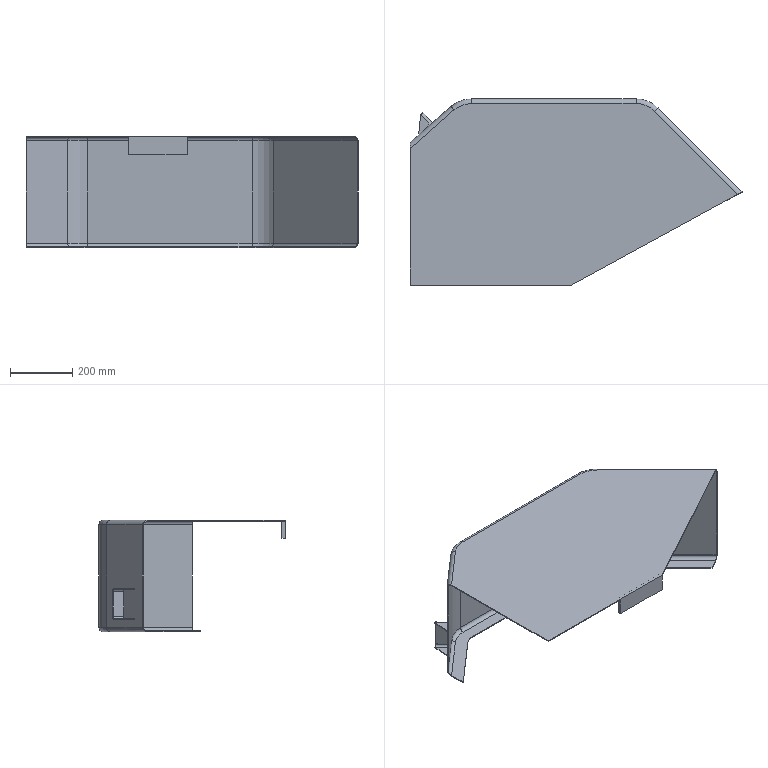Part | SolidWorks | 1 solid | 61 faces | box 1070 x 600 x 360 mm | volume 3106000 mm3 | plane 31 | cylinder 22 | torus 8 | commonest cylinder face diameters 24 x6 30 x6 14 x2 20 x2 90 x2 194 x2